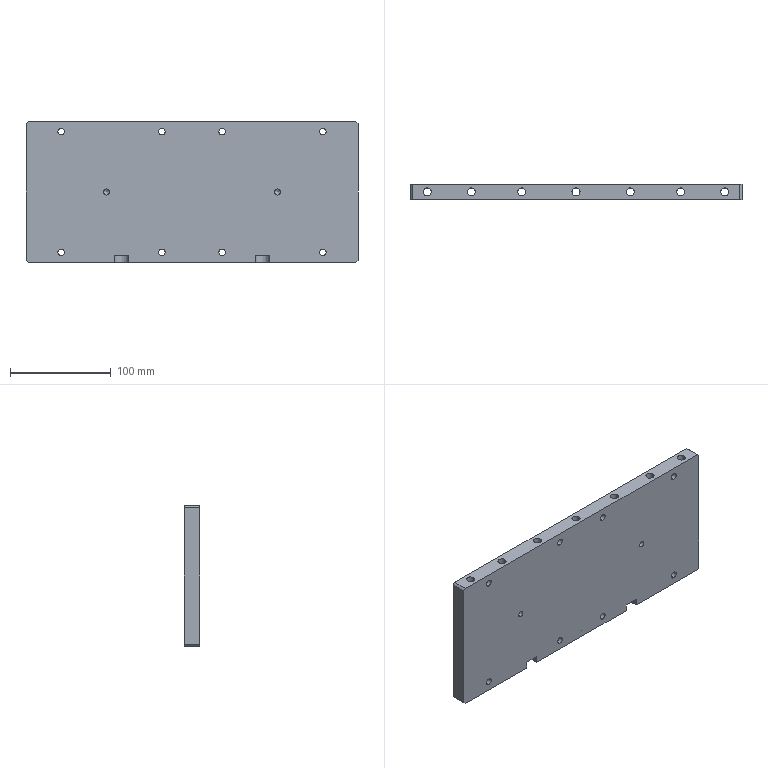Part | SolidWorks | features BaseBody 1 | 1 solid | 190 faces | box 330 x 15 x 140 mm | volume 619975 mm3 | cylinder 115 | cone 42 | plane 33 | commonest cylinder face diameters 8 x24 4.2 x16 6.6 x16 11 x16 3.3 x14 13 x11